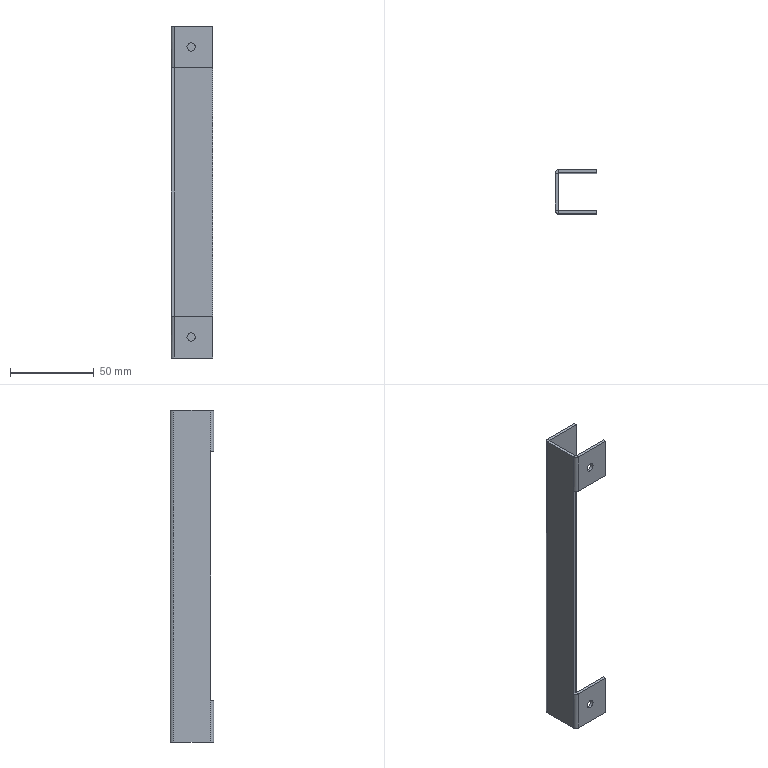Part | SolidWorks | features ICE 2, FlatPattern 1, SMBaseFlange 1, SheetMetal 1 | 1 solid | 34 faces | box 25 x 26 x 198 mm | volume 18838 mm3 | plane 26 | cylinder 8 | commonest cylinder face diameters 5 x4 0.4 x2 4 x2
STEP:
#1=CARTESIAN_POINT('',(-15.5,1.8,12.5));
#2=VERTEX_POINT('',#1);
#3=CARTESIAN_POINT('',(-10.5,1.8,12.5));
#4=VERTEX_POINT('',#3);
#5=CARTESIAN_POINT('',(-13.,1.8,12.5));
#6=DIRECTION('',(0.,-1.,0.));
#7=DIRECTION('',(1.,0.,0.));
#8=AXIS2_PLACEMENT_3D('',#5,#6,#7);
#9=CIRCLE('',#8,2.5);
#10=EDGE_CURVE('',#2,#4,#9,.T.);
#11=ORIENTED_EDGE('',*,*,#10,.F.);
#12=CARTESIAN_POINT('',(-15.5,0.,12.5));
#13=VERTEX_POINT('',#12);
#14=CARTESIAN_POINT('',(-15.5,10.,12.5));
#15=DIRECTION('',(0.,-1.,0.));
#16=VECTOR('',#15,1000.);
#17=LINE('',#14,#16);
#18=EDGE_CURVE('',#2,#13,#17,.T.);
#19=ORIENTED_EDGE('',*,*,#18,.T.);
#20=CARTESIAN_POINT('',(-10.5,0.,12.5));
#21=VERTEX_POINT('',#20);
#22=CARTESIAN_POINT('',(-13.,0.,12.5));
#23=DIRECTION('',(0.,-1.,0.));
#24=DIRECTION('',(1.,0.,0.));
#25=AXIS2_PLACEMENT_3D('',#22,#23,#24);
#26=CIRCLE('',#25,2.5);
#27=EDGE_CURVE('',#13,#21,#26,.T.);
#28=ORIENTED_EDGE('',*,*,#27,.T.);
#29=CARTESIAN_POINT('',(-10.5,10.,12.5));
#30=DIRECTION('',(0.,-1.,0.));
#31=VECTOR('',#30,1000.);
#32=LINE('',#29,#31);
#33=EDGE_CURVE('',#4,#21,#32,.T.);
#34=ORIENTED_EDGE('',*,*,#33,.F.);
#35=EDGE_LOOP('',(#11,#19,#28,#34));
#36=FACE_OUTER_BOUND('',#35,.T.);
#37=CARTESIAN_POINT('',(-13.,10.,12.5));
#38=DIRECTION('',(0.,-1.,0.));
#39=DIRECTION('',(1.,0.,0.));
#40=AXIS2_PLACEMENT_3D('',#37,#38,#39);
#41=CYLINDRICAL_SURFACE('',#40,2.5);
#42=ADVANCED_FACE('',(#36),#41,.F.);
#43=CARTESIAN_POINT('',(-15.5,1.8,185.5));
#44=VERTEX_POINT('',#43);
#45=CARTESIAN_POINT('',(-10.5,1.8,185.5));
#46=VERTEX_POINT('',#45);
#47=CARTESIAN_POINT('',(-13.,1.8,185.5));
#48=DIRECTION('',(0.,-1.,0.));
#49=DIRECTION('',(1.,0.,0.));
#50=AXIS2_PLACEMENT_3D('',#47,#48,#49);
#51=CIRCLE('',#50,2.5);
#52=EDGE_CURVE('',#44,#46,#51,.T.);
#53=ORIENTED_EDGE('',*,*,#52,.F.);
#54=CARTESIAN_POINT('',(-15.5,0.,185.5));
#55=VERTEX_POINT('',#54);
#56=CARTESIAN_POINT('',(-15.5,10.,185.5));
#57=DIRECTION('',(0.,-1.,0.));
#58=VECTOR('',#57,1000.);
#59=LINE('',#56,#58);
#60=EDGE_CURVE('',#44,#55,#59,.T.);
#61=ORIENTED_EDGE('',*,*,#60,.T.);
#62=CARTESIAN_POINT('',(-10.5,0.,185.5));
#63=VERTEX_POINT('',#62);
#64=CARTESIAN_POINT('',(-13.,0.,185.5));
#65=DIRECTION('',(0.,-1.,0.));
#66=DIRECTION('',(1.,0.,0.));
#67=AXIS2_PLACEMENT_3D('',#64,#65,#66);
#68=CIRCLE('',#67,2.5);
#69=EDGE_CURVE('',#55,#63,#68,.T.);
#70=ORIENTED_EDGE('',*,*,#69,.T.);
#71=CARTESIAN_POINT('',(-10.5,10.,185.5));
#72=DIRECTION('',(0.,-1.,0.));
#73=VECTOR('',#72,1000.);
#74=LINE('',#71,#73);
#75=EDGE_CURVE('',#46,#63,#74,.T.);
#76=ORIENTED_EDGE('',*,*,#75,.F.);
#77=EDGE_LOOP('',(#53,#61,#70,#76));
#78=FACE_OUTER_BOUND('',#77,.T.);
#79=CARTESIAN_POINT('',(-13.,10.,185.5));
#80=DIRECTION('',(0.,-1.,0.));
#81=DIRECTION('',(1.,0.,0.));
#82=AXIS2_PLACEMENT_3D('',#79,#80,#81);
#83=CYLINDRICAL_SURFACE('',#82,2.5);
#84=ADVANCED_FACE('',(#78),#83,.F.);
#85=CARTESIAN_POINT('',(-24.99,1.8,25.));
#86=VERTEX_POINT('',#85);
#87=CARTESIAN_POINT('',(-24.99,1.8,173.));
#88=VERTEX_POINT('',#87);
#89=CARTESIAN_POINT('',(-24.99,1.8,25.));
#90=DIRECTION('',(0.,0.,1.));
#91=VECTOR('',#90,1000.);
#92=LINE('',#89,#91);
#93=EDGE_CURVE('',#86,#88,#92,.T.);
#94=ORIENTED_EDGE('',*,*,#93,.T.);
#95=CARTESIAN_POINT('',(-23.,0.,173.));
#96=VERTEX_POINT('',#95);
#97=CARTESIAN_POINT('',(-23.,2.,173.));
#98=DIRECTION('',(0.,0.,1.));
#99=DIRECTION('',(1.,0.,0.));
#100=AXIS2_PLACEMENT_3D('',#97,#98,#99);
#101=CIRCLE('',#100,2.);
#102=EDGE_CURVE('',#88,#96,#101,.T.);
#103=ORIENTED_EDGE('',*,*,#102,.T.);
#104=CARTESIAN_POINT('',(-23.,0.,198.));
#105=VERTEX_POINT('',#104);
#106=CARTESIAN_POINT('',(-23.,0.,198.));
#107=DIRECTION('',(0.,0.,-1.));
#108=VECTOR('',#107,1000.);
#109=LINE('',#106,#108);
#110=EDGE_CURVE('',#105,#96,#109,.T.);
#111=ORIENTED_EDGE('',*,*,#110,.F.);
#112=CARTESIAN_POINT('',(-25.,2.,198.));
#113=VERTEX_POINT('',#112);
#114=CARTESIAN_POINT('',(-23.,2.,198.));
#115=DIRECTION('',(0.,0.,-1.));
#116=DIRECTION('',(1.,0.,0.));
#117=AXIS2_PLACEMENT_3D('',#114,#115,#116);
#118=CIRCLE('',#117,2.);
#119=EDGE_CURVE('',#105,#113,#118,.T.);
#120=ORIENTED_EDGE('',*,*,#119,.T.);
#121=CARTESIAN_POINT('',(-25.,2.,0.));
#122=VERTEX_POINT('',#121);
#123=CARTESIAN_POINT('',(-25.,2.,198.));
#124=DIRECTION('',(0.,0.,-1.));
#125=VECTOR('',#124,1000.);
#126=LINE('',#123,#125);
#127=EDGE_CURVE('',#113,#122,#126,.T.);
#128=ORIENTED_EDGE('',*,*,#127,.T.);
#129=CARTESIAN_POINT('',(-23.,0.,0.));
#130=VERTEX_POINT('',#129);
#131=CARTESIAN_POINT('',(-23.,2.,0.));
#132=DIRECTION('',(0.,0.,-1.));
#133=DIRECTION('',(1.,0.,0.));
#134=AXIS2_PLACEMENT_3D('',#131,#132,#133);
#135=CIRCLE('',#134,2.);
#136=EDGE_CURVE('',#130,#122,#135,.T.);
#137=ORIENTED_EDGE('',*,*,#136,.F.);
#138=CARTESIAN_POINT('',(-23.,0.,25.));
#139=VERTEX_POINT('',#138);
#140=CARTESIAN_POINT('',(-23.,0.,198.));
#141=DIRECTION('',(0.,0.,-1.));
#142=VECTOR('',#141,1000.);
#143=LINE('',#140,#142);
#144=EDGE_CURVE('',#139,#130,#143,.T.);
#145=ORIENTED_EDGE('',*,*,#144,.F.);
#146=CARTESIAN_POINT('',(-23.,2.,25.));
#147=DIRECTION('',(0.,0.,-1.));
#148=DIRECTION('',(-1.,0.,0.));
#149=AXIS2_PLACEMENT_3D('',#146,#147,#148);
#150=CIRCLE('',#149,2.);
#151=EDGE_CURVE('',#139,#86,#150,.T.);
#152=ORIENTED_EDGE('',*,*,#151,.T.);
#153=EDGE_LOOP('',(#94,#103,#111,#120,#128,#137,#145,#152));
#154=FACE_OUTER_BOUND('',#153,.T.);
#155=CARTESIAN_POINT('',(-23.,2.,198.));
#156=DIRECTION('',(0.,0.,-1.));
#157=DIRECTION('',(-1.,0.,0.));
#158=AXIS2_PLACEMENT_3D('',#155,#156,#157);
#159=CYLINDRICAL_SURFACE('',#158,2.);
#160=ADVANCED_FACE('',(#154),#159,.T.);
#161=CARTESIAN_POINT('',(-13.,0.,12.5));
#162=DIRECTION('',(0.,-1.,0.));
#163=DIRECTION('',(1.,0.,0.));
#164=AXIS2_PLACEMENT_3D('',#161,#162,#163);
#165=CIRCLE('',#164,2.5);
#166=EDGE_CURVE('',#21,#13,#165,.T.);
#167=ORIENTED_EDGE('',*,*,#166,.F.);
#168=ORIENTED_EDGE('',*,*,#27,.F.);
#169=EDGE_LOOP('',(#167,#168));
#170=FACE_BOUND('',#169,.T.);
#171=CARTESIAN_POINT('',(0.,0.,25.));
#172=VERTEX_POINT('',#171);
#173=CARTESIAN_POINT('',(0.,0.,0.));
#174=VERTEX_POINT('',#173);
#175=CARTESIAN_POINT('',(0.,0.,198.));
#176=DIRECTION('',(0.,0.,-1.));
#177=VECTOR('',#176,1000.);
#178=LINE('',#175,#177);
#179=EDGE_CURVE('',#172,#174,#178,.T.);
#180=ORIENTED_EDGE('',*,*,#179,.F.);
#181=CARTESIAN_POINT('',(45.,0.,25.));
#182=DIRECTION('',(1.,0.,0.));
#183=VECTOR('',#182,1000.);
#184=LINE('',#181,#183);
#185=EDGE_CURVE('',#139,#172,#184,.T.);
#186=ORIENTED_EDGE('',*,*,#185,.F.);
#187=ORIENTED_EDGE('',*,*,#144,.T.);
#188=CARTESIAN_POINT('',(0.,0.,0.));
#189=DIRECTION('',(-1.,0.,0.));
#190=VECTOR('',#189,1000.);
#191=LINE('',#188,#190);
#192=EDGE_CURVE('',#174,#130,#191,.T.);
#193=ORIENTED_EDGE('',*,*,#192,.F.);
#194=EDGE_LOOP('',(#180,#186,#187,#193));
#195=FACE_OUTER_BOUND('',#194,.T.);
#196=CARTESIAN_POINT('',(0.,0.,198.));
#197=DIRECTION('',(0.,-1.,0.));
#198=DIRECTION('',(1.,0.,0.));
#199=AXIS2_PLACEMENT_3D('',#196,#197,#198);
#200=PLANE('',#199);
#201=ADVANCED_FACE('',(#170,#195),#200,.T.);
#202=CARTESIAN_POINT('',(-13.,0.,185.5));
#203=DIRECTION('',(0.,-1.,0.));
#204=DIRECTION('',(1.,0.,0.));
#205=AXIS2_PLACEMENT_3D('',#202,#203,#204);
#206=CIRCLE('',#205,2.5);
#207=EDGE_CURVE('',#63,#55,#206,.T.);
#208=ORIENTED_EDGE('',*,*,#207,.F.);
#209=ORIENTED_EDGE('',*,*,#69,.F.);
#210=EDGE_LOOP('',(#208,#209));
#211=FACE_BOUND('',#210,.T.);
#212=ORIENTED_EDGE('',*,*,#110,.T.);
#213=CARTESIAN_POINT('',(0.,0.,173.));
#214=VERTEX_POINT('',#213);
#215=CARTESIAN_POINT('',(45.,0.,173.));
#216=DIRECTION('',(-1.,0.,0.));
#217=VECTOR('',#216,1000.);
#218=LINE('',#215,#217);
#219=EDGE_CURVE('',#214,#96,#218,.T.);
#220=ORIENTED_EDGE('',*,*,#219,.F.);
#221=CARTESIAN_POINT('',(0.,0.,198.));
#222=VERTEX_POINT('',#221);
#223=CARTESIAN_POINT('',(0.,0.,198.));
#224=DIRECTION('',(0.,0.,-1.));
#225=VECTOR('',#224,1000.);
#226=LINE('',#223,#225);
#227=EDGE_CURVE('',#222,#214,#226,.T.);
#228=ORIENTED_EDGE('',*,*,#227,.F.);
#229=CARTESIAN_POINT('',(0.,0.,198.));
#230=DIRECTION('',(-1.,0.,0.));
#231=VECTOR('',#230,1000.);
#232=LINE('',#229,#231);
#233=EDGE_CURVE('',#222,#105,#232,.T.);
#234=ORIENTED_EDGE('',*,*,#233,.T.);
#235=EDGE_LOOP('',(#212,#220,#228,#234));
#236=FACE_OUTER_BOUND('',#235,.T.);
#237=CARTESIAN_POINT('',(0.,0.,198.));
#238=DIRECTION('',(0.,-1.,0.));
#239=DIRECTION('',(1.,0.,0.));
#240=AXIS2_PLACEMENT_3D('',#237,#238,#239);
#241=PLANE('',#240);
#242=ADVANCED_FACE('',(#211,#236),#241,.T.);
#243=CARTESIAN_POINT('',(0.,1.8,25.));
#244=VERTEX_POINT('',#243);
#245=CARTESIAN_POINT('',(0.,1.8,0.));
#246=VERTEX_POINT('',#245);
#247=CARTESIAN_POINT('',(0.,1.8,198.));
#248=DIRECTION('',(0.,0.,-1.));
#249=VECTOR('',#248,1000.);
#250=LINE('',#247,#249);
#251=EDGE_CURVE('',#244,#246,#250,.T.);
#252=ORIENTED_EDGE('',*,*,#251,.F.);
#253=CARTESIAN_POINT('',(0.,0.,25.));
#254=DIRECTION('',(0.,1.,0.));
#255=VECTOR('',#254,1000.);
#256=LINE('',#253,#255);
#257=EDGE_CURVE('',#172,#244,#256,.T.);
#258=ORIENTED_EDGE('',*,*,#257,.F.);
#259=ORIENTED_EDGE('',*,*,#179,.T.);
#260=CARTESIAN_POINT('',(0.,1.8,0.));
#261=DIRECTION('',(0.,-1.,0.));
#262=VECTOR('',#261,1000.);
#263=LINE('',#260,#262);
#264=EDGE_CURVE('',#246,#174,#263,.T.);
#265=ORIENTED_EDGE('',*,*,#264,.F.);
#266=EDGE_LOOP('',(#252,#258,#259,#265));
#267=FACE_OUTER_BOUND('',#266,.T.);
#268=CARTESIAN_POINT('',(0.,1.8,198.));
#269=DIRECTION('',(1.,0.,0.));
#270=DIRECTION('',(0.,1.,0.));
#271=AXIS2_PLACEMENT_3D('',#268,#269,#270);
#272=PLANE('',#271);
#273=ADVANCED_FACE('',(#267),#272,.T.);
#274=ORIENTED_EDGE('',*,*,#227,.T.);
#275=CARTESIAN_POINT('',(0.,1.8,173.));
#276=VERTEX_POINT('',#275);
#277=CARTESIAN_POINT('',(0.,0.,173.));
#278=DIRECTION('',(0.,1.,0.));
#279=VECTOR('',#278,1000.);
#280=LINE('',#277,#279);
#281=EDGE_CURVE('',#214,#276,#280,.T.);
#282=ORIENTED_EDGE('',*,*,#281,.T.);
#283=CARTESIAN_POINT('',(0.,1.8,198.));
#284=VERTEX_POINT('',#283);
#285=CARTESIAN_POINT('',(0.,1.8,198.));
#286=DIRECTION('',(0.,0.,-1.));
#287=VECTOR('',#286,1000.);
#288=LINE('',#285,#287);
#289=EDGE_CURVE('',#284,#276,#288,.T.);
#290=ORIENTED_EDGE('',*,*,#289,.F.);
#291=CARTESIAN_POINT('',(0.,1.8,198.));
#292=DIRECTION('',(0.,-1.,0.));
#293=VECTOR('',#292,1000.);
#294=LINE('',#291,#293);
#295=EDGE_CURVE('',#284,#222,#294,.T.);
#296=ORIENTED_EDGE('',*,*,#295,.T.);
#297=EDGE_LOOP('',(#274,#282,#290,#296));
#298=FACE_OUTER_BOUND('',#297,.T.);
#299=CARTESIAN_POINT('',(0.,1.8,198.));
#300=DIRECTION('',(1.,0.,0.));
#301=DIRECTION('',(0.,1.,0.));
#302=AXIS2_PLACEMENT_3D('',#299,#300,#301);
#303=PLANE('',#302);
#304=ADVANCED_FACE('',(#298),#303,.T.);
#305=CARTESIAN_POINT('',(-13.,1.8,12.5));
#306=DIRECTION('',(0.,-1.,0.));
#307=DIRECTION('',(1.,0.,0.));
#308=AXIS2_PLACEMENT_3D('',#305,#306,#307);
#309=CIRCLE('',#308,2.5);
#310=EDGE_CURVE('',#4,#2,#309,.T.);
#311=ORIENTED_EDGE('',*,*,#310,.T.);
#312=ORIENTED_EDGE('',*,*,#10,.T.);
#313=EDGE_LOOP('',(#311,#312));
#314=FACE_BOUND('',#313,.T.);
#315=CARTESIAN_POINT('',(-23.,1.8,25.));
#316=VERTEX_POINT('',#315);
#317=CARTESIAN_POINT('',(0.,1.8,25.));
#318=DIRECTION('',(1.,0.,0.));
#319=VECTOR('',#318,1000.);
#320=LINE('',#317,#319);
#321=EDGE_CURVE('',#316,#244,#320,.T.);
#322=ORIENTED_EDGE('',*,*,#321,.T.);
#323=ORIENTED_EDGE('',*,*,#251,.T.);
#324=CARTESIAN_POINT('',(-23.,1.8,0.));
#325=VERTEX_POINT('',#324);
#326=CARTESIAN_POINT('',(0.,1.8,0.));
#327=DIRECTION('',(-1.,0.,0.));
#328=VECTOR('',#327,1000.);
#329=LINE('',#326,#328);
#330=EDGE_CURVE('',#246,#325,#329,.T.);
#331=ORIENTED_EDGE('',*,*,#330,.T.);
#332=CARTESIAN_POINT('',(-23.,1.8,198.));
#333=DIRECTION('',(0.,0.,-1.));
#334=VECTOR('',#333,1000.);
#335=LINE('',#332,#334);
#336=EDGE_CURVE('',#316,#325,#335,.T.);
#337=ORIENTED_EDGE('',*,*,#336,.F.);
#338=EDGE_LOOP('',(#322,#323,#331,#337));
#339=FACE_OUTER_BOUND('',#338,.T.);
#340=CARTESIAN_POINT('',(0.,1.8,198.));
#341=DIRECTION('',(0.,-1.,0.));
#342=DIRECTION('',(1.,0.,0.));
#343=AXIS2_PLACEMENT_3D('',#340,#341,#342);
#344=PLANE('',#343);
#345=ADVANCED_FACE('',(#314,#339),#344,.F.);
#346=CARTESIAN_POINT('',(-13.,1.8,185.5));
#347=DIRECTION('',(0.,-1.,0.));
#348=DIRECTION('',(1.,0.,0.));
#349=AXIS2_PLACEMENT_3D('',#346,#347,#348);
#350=CIRCLE('',#349,2.5);
#351=EDGE_CURVE('',#46,#44,#350,.T.);
#352=ORIENTED_EDGE('',*,*,#351,.T.);
#353=ORIENTED_EDGE('',*,*,#52,.T.);
#354=EDGE_LOOP('',(#352,#353));
#355=FACE_BOUND('',#354,.T.);
#356=CARTESIAN_POINT('',(-23.,1.8,173.));
#357=VERTEX_POINT('',#356);
#358=CARTESIAN_POINT('',(0.,1.8,173.));
#359=DIRECTION('',(-1.,0.,0.));
#360=VECTOR('',#359,1000.);
#361=LINE('',#358,#360);
#362=EDGE_CURVE('',#276,#357,#361,.T.);
#363=ORIENTED_EDGE('',*,*,#362,.T.);
#364=CARTESIAN_POINT('',(-23.,1.8,198.));
#365=VERTEX_POINT('',#364);
#366=CARTESIAN_POINT('',(-23.,1.8,198.));
#367=DIRECTION('',(0.,0.,-1.));
#368=VECTOR('',#367,1000.);
#369=LINE('',#366,#368);
#370=EDGE_CURVE('',#365,#357,#369,.T.);
#371=ORIENTED_EDGE('',*,*,#370,.F.);
#372=CARTESIAN_POINT('',(0.,1.8,198.));
#373=DIRECTION('',(-1.,0.,0.));
#374=VECTOR('',#373,1000.);
#375=LINE('',#372,#374);
#376=EDGE_CURVE('',#284,#365,#375,.T.);
#377=ORIENTED_EDGE('',*,*,#376,.F.);
#378=ORIENTED_EDGE('',*,*,#289,.T.);
#379=EDGE_LOOP('',(#363,#371,#377,#378));
#380=FACE_OUTER_BOUND('',#379,.T.);
#381=CARTESIAN_POINT('',(0.,1.8,198.));
#382=DIRECTION('',(0.,-1.,0.));
#383=DIRECTION('',(1.,0.,0.));
#384=AXIS2_PLACEMENT_3D('',#381,#382,#383);
#385=PLANE('',#384);
#386=ADVANCED_FACE('',(#355,#380),#385,.F.);
#387=CARTESIAN_POINT('',(-23.199,1.98,173.));
#388=VERTEX_POINT('',#387);
#389=CARTESIAN_POINT('',(-23.,2.,173.));
#390=DIRECTION('',(0.,0.,1.));
#391=DIRECTION('',(-1.,0.,0.));
#392=AXIS2_PLACEMENT_3D('',#389,#390,#391);
#393=CIRCLE('',#392,0.2);
#394=EDGE_CURVE('',#388,#357,#393,.T.);
#395=ORIENTED_EDGE('',*,*,#394,.F.);
#396=CARTESIAN_POINT('',(-23.199,1.98,25.));
#397=VERTEX_POINT('',#396);
#398=CARTESIAN_POINT('',(-23.199,1.98,210.51));
#399=DIRECTION('',(0.,0.,1.));
#400=VECTOR('',#399,1000.);
#401=LINE('',#398,#400);
#402=EDGE_CURVE('',#397,#388,#401,.T.);
#403=ORIENTED_EDGE('',*,*,#402,.F.);
#404=CARTESIAN_POINT('',(-23.,2.,25.));
#405=DIRECTION('',(0.,0.,-1.));
#406=DIRECTION('',(-1.,0.,0.));
#407=AXIS2_PLACEMENT_3D('',#404,#405,#406);
#408=CIRCLE('',#407,0.2);
#409=EDGE_CURVE('',#316,#397,#408,.T.);
#410=ORIENTED_EDGE('',*,*,#409,.F.);
#411=ORIENTED_EDGE('',*,*,#336,.T.);
#412=CARTESIAN_POINT('',(-23.2,2.,0.));
#413=VERTEX_POINT('',#412);
#414=CARTESIAN_POINT('',(-23.,2.,0.));
#415=DIRECTION('',(0.,0.,-1.));
#416=DIRECTION('',(1.,0.,0.));
#417=AXIS2_PLACEMENT_3D('',#414,#415,#416);
#418=CIRCLE('',#417,0.2);
#419=EDGE_CURVE('',#325,#413,#418,.T.);
#420=ORIENTED_EDGE('',*,*,#419,.T.);
#421=CARTESIAN_POINT('',(-23.2,2.,198.));
#422=VERTEX_POINT('',#421);
#423=CARTESIAN_POINT('',(-23.2,2.,198.));
#424=DIRECTION('',(0.,0.,-1.));
#425=VECTOR('',#424,1000.);
#426=LINE('',#423,#425);
#427=EDGE_CURVE('',#422,#413,#426,.T.);
#428=ORIENTED_EDGE('',*,*,#427,.F.);
#429=CARTESIAN_POINT('',(-23.,2.,198.));
#430=DIRECTION('',(0.,0.,-1.));
#431=DIRECTION('',(1.,0.,0.));
#432=AXIS2_PLACEMENT_3D('',#429,#430,#431);
#433=CIRCLE('',#432,0.2);
#434=EDGE_CURVE('',#365,#422,#433,.T.);
#435=ORIENTED_EDGE('',*,*,#434,.F.);
#436=ORIENTED_EDGE('',*,*,#370,.T.);
#437=EDGE_LOOP('',(#395,#403,#410,#411,#420,#428,#435,#436));
#438=FACE_OUTER_BOUND('',#437,.T.);
#439=CARTESIAN_POINT('',(-23.,2.,198.));
#440=DIRECTION('',(0.,0.,-1.));
#441=DIRECTION('',(-1.,0.,0.));
#442=AXIS2_PLACEMENT_3D('',#439,#440,#441);
#443=CYLINDRICAL_SURFACE('',#442,0.2);
#444=ADVANCED_FACE('',(#438),#443,.F.);
#445=CARTESIAN_POINT('',(-25.,2.,198.));
#446=DIRECTION('',(1.,0.,0.));
#447=VECTOR('',#446,1000.);
#448=LINE('',#445,#447);
#449=EDGE_CURVE('',#113,#422,#448,.T.);
#450=ORIENTED_EDGE('',*,*,#449,.F.);
#451=ORIENTED_EDGE('',*,*,#119,.F.);
#452=CARTESIAN_POINT('',(-23.,1.8,198.));
#453=DIRECTION('',(0.,-1.,0.));
#454=VECTOR('',#453,1000.);
#455=LINE('',#452,#454);
#456=EDGE_CURVE('',#365,#105,#455,.T.);
#457=ORIENTED_EDGE('',*,*,#456,.F.);
#458=ORIENTED_EDGE('',*,*,#434,.T.);
#459=EDGE_LOOP('',(#450,#451,#457,#458));
#460=FACE_OUTER_BOUND('',#459,.T.);
#461=CARTESIAN_POINT('',(-25.,2.,198.));
#462=DIRECTION('',(0.,0.,1.));
#463=DIRECTION('',(1.,0.,0.));
#464=AXIS2_PLACEMENT_3D('',#461,#462,#463);
#465=PLANE('',#464);
#466=ADVANCED_FACE('',(#460),#465,.T.);
#467=CARTESIAN_POINT('',(-25.,24.,198.));
#468=VERTEX_POINT('',#467);
#469=CARTESIAN_POINT('',(-25.,0.,198.));
#470=DIRECTION('',(0.,1.,0.));
#471=VECTOR('',#470,1000.);
#472=LINE('',#469,#471);
#473=EDGE_CURVE('',#113,#468,#472,.T.);
#474=ORIENTED_EDGE('',*,*,#473,.F.);
#475=ORIENTED_EDGE('',*,*,#449,.T.);
#476=CARTESIAN_POINT('',(-23.2,24.,198.));
#477=VERTEX_POINT('',#476);
#478=CARTESIAN_POINT('',(-23.2,0.,198.));
#479=DIRECTION('',(0.,1.,0.));
#480=VECTOR('',#479,1000.);
#481=LINE('',#478,#480);
#482=EDGE_CURVE('',#422,#477,#481,.T.);
#483=ORIENTED_EDGE('',*,*,#482,.T.);
#484=CARTESIAN_POINT('',(-23.2,24.,198.));
#485=DIRECTION('',(-1.,0.,0.));
#486=VECTOR('',#485,1000.);
#487=LINE('',#484,#486);
#488=EDGE_CURVE('',#477,#468,#487,.T.);
#489=ORIENTED_EDGE('',*,*,#488,.T.);
#490=EDGE_LOOP('',(#474,#475,#483,#489));
#491=FACE_OUTER_BOUND('',#490,.T.);
#492=CARTESIAN_POINT('',(-23.,1.8,198.));
#493=DIRECTION('',(0.,0.,1.));
#494=DIRECTION('',(1.,0.,0.));
#495=AXIS2_PLACEMENT_3D('',#492,#493,#494);
#496=PLANE('',#495);
#497=ADVANCED_FACE('',(#491),#496,.T.);
#498=CARTESIAN_POINT('',(-23.,0.,0.));
#499=DIRECTION('',(0.,1.,0.));
#500=VECTOR('',#499,1000.);
#501=LINE('',#498,#500);
#502=EDGE_CURVE('',#130,#325,#501,.T.);
#503=ORIENTED_EDGE('',*,*,#502,.F.);
#504=ORIENTED_EDGE('',*,*,#136,.T.);
#505=CARTESIAN_POINT('',(-23.2,2.,0.));
#506=DIRECTION('',(-1.,0.,0.));
#507=VECTOR('',#506,1000.);
#508=LINE('',#505,#507);
#509=EDGE_CURVE('',#413,#122,#508,.T.);
#510=ORIENTED_EDGE('',*,*,#509,.F.);
#511=ORIENTED_EDGE('',*,*,#419,.F.);
#512=EDGE_LOOP('',(#503,#504,#510,#511));
#513=FACE_OUTER_BOUND('',#512,.T.);
#514=CARTESIAN_POINT('',(-23.,0.,0.));
#515=DIRECTION('',(0.,0.,-1.));
#516=DIRECTION('',(-1.,0.,0.));
#517=AXIS2_PLACEMENT_3D('',#514,#515,#516);
#518=PLANE('',#517);
#519=ADVANCED_FACE('',(#513),#518,.T.);
#520=ORIENTED_EDGE('',*,*,#192,.T.);
#521=ORIENTED_EDGE('',*,*,#502,.T.);
#522=ORIENTED_EDGE('',*,*,#330,.F.);
#523=ORIENTED_EDGE('',*,*,#264,.T.);
#524=EDGE_LOOP('',(#520,#521,#522,#523));
#525=FACE_OUTER_BOUND('',#524,.T.);
#526=CARTESIAN_POINT('',(-23.2,2.,0.));
#527=DIRECTION('',(0.,0.,-1.));
#528=DIRECTION('',(-1.,0.,0.));
#529=AXIS2_PLACEMENT_3D('',#526,#527,#528);
#530=PLANE('',#529);
#531=ADVANCED_FACE('',(#525),#530,.T.);
#532=CARTESIAN_POINT('',(-23.,26.,198.));
#533=VERTEX_POINT('',#532);
#534=CARTESIAN_POINT('',(-23.,24.2,198.));
#535=VERTEX_POINT('',#534);
#536=CARTESIAN_POINT('',(-23.,26.,198.));
#537=DIRECTION('',(0.,-1.,0.));
#538=VECTOR('',#537,1000.);
#539=LINE('',#536,#538);
#540=EDGE_CURVE('',#533,#535,#539,.T.);
#541=ORIENTED_EDGE('',*,*,#540,.F.);
#542=CARTESIAN_POINT('',(-23.,24.,198.));
#543=DIRECTION('',(0.,0.,-1.));
#544=DIRECTION('',(1.,0.,0.));
#545=AXIS2_PLACEMENT_3D('',#542,#543,#544);
#546=CIRCLE('',#545,2.);
#547=EDGE_CURVE('',#468,#533,#546,.T.);
#548=ORIENTED_EDGE('',*,*,#547,.F.);
#549=ORIENTED_EDGE('',*,*,#488,.F.);
#550=CARTESIAN_POINT('',(-23.,24.,198.));
#551=DIRECTION('',(0.,0.,-1.));
#552=DIRECTION('',(1.,0.,0.));
#553=AXIS2_PLACEMENT_3D('',#550,#551,#552);
#554=CIRCLE('',#553,0.2);
#555=EDGE_CURVE('',#477,#535,#554,.T.);
#556=ORIENTED_EDGE('',*,*,#555,.T.);
#557=EDGE_LOOP('',(#541,#548,#549,#556));
#558=FACE_OUTER_BOUND('',#557,.T.);
#559=CARTESIAN_POINT('',(-23.,26.,198.));
#560=DIRECTION('',(0.,0.,1.));
#561=DIRECTION('',(1.,0.,0.));
#562=AXIS2_PLACEMENT_3D('',#559,#560,#561);
#563=PLANE('',#562);
#564=ADVANCED_FACE('',(#558),#563,.T.);
#565=CARTESIAN_POINT('',(0.,26.,198.));
#566=VERTEX_POINT('',#565);
#567=CARTESIAN_POINT('',(-25.,26.,198.));
#568=DIRECTION('',(1.,0.,0.));
#569=VECTOR('',#568,1000.);
#570=LINE('',#567,#569);
#571=EDGE_CURVE('',#533,#566,#570,.T.);
#572=ORIENTED_EDGE('',*,*,#571,.F.);
#573=ORIENTED_EDGE('',*,*,#540,.T.);
#574=CARTESIAN_POINT('',(0.,24.2,198.));
#575=VERTEX_POINT('',#574);
#576=CARTESIAN_POINT('',(-25.,24.2,198.));
#577=DIRECTION('',(1.,0.,0.));
#578=VECTOR('',#577,1000.);
#579=LINE('',#576,#578);
#580=EDGE_CURVE('',#535,#575,#579,.T.);
#581=ORIENTED_EDGE('',*,*,#580,.T.);
#582=CARTESIAN_POINT('',(0.,26.,198.));
#583=DIRECTION('',(0.,-1.,0.));
#584=VECTOR('',#583,1000.);
#585=LINE('',#582,#584);
#586=EDGE_CURVE('',#566,#575,#585,.T.);
#587=ORIENTED_EDGE('',*,*,#586,.F.);
#588=EDGE_LOOP('',(#572,#573,#581,#587));
#589=FACE_OUTER_BOUND('',#588,.T.);
#590=CARTESIAN_POINT('',(-23.2,24.,198.));
#591=DIRECTION('',(0.,0.,1.));
#592=DIRECTION('',(1.,0.,0.));
#593=AXIS2_PLACEMENT_3D('',#590,#591,#592);
#594=PLANE('',#593);
#595=ADVANCED_FACE('',(#589),#594,.T.);
#596=CARTESIAN_POINT('',(-25.,24.,0.));
#597=VERTEX_POINT('',#596);
#598=CARTESIAN_POINT('',(-23.2,24.,0.));
#599=VERTEX_POINT('',#598);
#600=CARTESIAN_POINT('',(-25.,24.,0.));
#601=DIRECTION('',(1.,0.,0.));
#602=VECTOR('',#601,1000.);
#603=LINE('',#600,#602);
#604=EDGE_CURVE('',#597,#599,#603,.T.);
#605=ORIENTED_EDGE('',*,*,#604,.F.);
#606=CARTESIAN_POINT('',(-23.,26.,0.));
#607=VERTEX_POINT('',#606);
#608=CARTESIAN_POINT('',(-23.,24.,0.));
#609=DIRECTION('',(0.,0.,-1.));
#610=DIRECTION('',(1.,0.,0.));
#611=AXIS2_PLACEMENT_3D('',#608,#609,#610);
#612=CIRCLE('',#611,2.);
#613=EDGE_CURVE('',#597,#607,#612,.T.);
#614=ORIENTED_EDGE('',*,*,#613,.T.);
#615=CARTESIAN_POINT('',(-23.,24.2,0.));
#616=VERTEX_POINT('',#615);
#617=CARTESIAN_POINT('',(-23.,24.2,0.));
#618=DIRECTION('',(0.,1.,0.));
#619=VECTOR('',#618,1000.);
#620=LINE('',#617,#619);
#621=EDGE_CURVE('',#616,#607,#620,.T.);
#622=ORIENTED_EDGE('',*,*,#621,.F.);
#623=CARTESIAN_POINT('',(-23.,24.,0.));
#624=DIRECTION('',(0.,0.,-1.));
#625=DIRECTION('',(1.,0.,0.));
#626=AXIS2_PLACEMENT_3D('',#623,#624,#625);
#627=CIRCLE('',#626,0.2);
#628=EDGE_CURVE('',#599,#616,#627,.T.);
#629=ORIENTED_EDGE('',*,*,#628,.F.);
#630=EDGE_LOOP('',(#605,#614,#622,#629));
#631=FACE_OUTER_BOUND('',#630,.T.);
#632=CARTESIAN_POINT('',(-25.,24.,0.));
#633=DIRECTION('',(0.,0.,-1.));
#634=DIRECTION('',(-1.,0.,0.));
#635=AXIS2_PLACEMENT_3D('',#632,#633,#634);
#636=PLANE('',#635);
#637=ADVANCED_FACE('',(#631),#636,.T.);
#638=CARTESIAN_POINT('',(-25.,0.,0.));
#639=DIRECTION('',(0.,1.,0.));
#640=VECTOR('',#639,1000.);
#641=LINE('',#638,#640);
#642=EDGE_CURVE('',#122,#597,#641,.T.);
#643=ORIENTED_EDGE('',*,*,#642,.T.);
#644=ORIENTED_EDGE('',*,*,#604,.T.);
#645=CARTESIAN_POINT('',(-23.2,0.,0.));
#646=DIRECTION('',(0.,1.,0.));
#647=VECTOR('',#646,1000.);
#648=LINE('',#645,#647);
#649=EDGE_CURVE('',#413,#599,#648,.T.);
#650=ORIENTED_EDGE('',*,*,#649,.F.);
#651=ORIENTED_EDGE('',*,*,#509,.T.);
#652=EDGE_LOOP('',(#643,#644,#650,#651));
#653=FACE_OUTER_BOUND('',#652,.T.);
#654=CARTESIAN_POINT('',(-23.,24.2,0.));
#655=DIRECTION('',(0.,0.,-1.));
#656=DIRECTION('',(-1.,0.,0.));
#657=AXIS2_PLACEMENT_3D('',#654,#655,#656);
#658=PLANE('',#657);
#659=ADVANCED_FACE('',(#653),#658,.T.);
#660=CARTESIAN_POINT('',(0.,24.2,0.));
#661=VERTEX_POINT('',#660);
#662=CARTESIAN_POINT('',(-25.,24.2,0.));
#663=DIRECTION('',(1.,0.,0.));
#664=VECTOR('',#663,1000.);
#665=LINE('',#662,#664);
#666=EDGE_CURVE('',#616,#661,#665,.T.);
#667=ORIENTED_EDGE('',*,*,#666,.T.);
#668=CARTESIAN_POINT('',(0.,24.2,198.));
#669=DIRECTION('',(0.,0.,-1.));
#670=VECTOR('',#669,1000.);
#671=LINE('',#668,#670);
#672=EDGE_CURVE('',#575,#661,#671,.T.);
#673=ORIENTED_EDGE('',*,*,#672,.F.);
#674=ORIENTED_EDGE('',*,*,#580,.F.);
#675=CARTESIAN_POINT('',(-23.,24.2,198.));
#676=DIRECTION('',(0.,0.,-1.));
#677=VECTOR('',#676,1000.);
#678=LINE('',#675,#677);
#679=EDGE_CURVE('',#535,#616,#678,.T.);
#680=ORIENTED_EDGE('',*,*,#679,.T.);
#681=EDGE_LOOP('',(#667,#673,#674,#680));
#682=FACE_OUTER_BOUND('',#681,.T.);
#683=CARTESIAN_POINT('',(-25.,24.2,198.));
#684=DIRECTION('',(0.,1.,0.));
#685=DIRECTION('',(-1.,0.,0.));
#686=AXIS2_PLACEMENT_3D('',#683,#684,#685);
#687=PLANE('',#686);
#688=ADVANCED_FACE('',(#682),#687,.F.);
#689=CARTESIAN_POINT('',(0.,26.,0.));
#690=VERTEX_POINT('',#689);
#691=CARTESIAN_POINT('',(0.,26.,0.));
#692=DIRECTION('',(0.,-1.,0.));
#693=VECTOR('',#692,1000.);
#694=LINE('',#691,#693);
#695=EDGE_CURVE('',#690,#661,#694,.T.);
#696=ORIENTED_EDGE('',*,*,#695,.F.);
#697=CARTESIAN_POINT('',(0.,26.,198.));
#698=DIRECTION('',(0.,0.,-1.));
#699=VECTOR('',#698,1000.);
#700=LINE('',#697,#699);
#701=EDGE_CURVE('',#566,#690,#700,.T.);
#702=ORIENTED_EDGE('',*,*,#701,.F.);
#703=ORIENTED_EDGE('',*,*,#586,.T.);
#704=ORIENTED_EDGE('',*,*,#672,.T.);
#705=EDGE_LOOP('',(#696,#702,#703,#704));
#706=FACE_OUTER_BOUND('',#705,.T.);
#707=CARTESIAN_POINT('',(0.,26.,198.));
#708=DIRECTION('',(1.,0.,0.));
#709=DIRECTION('',(0.,0.,-1.));
#710=AXIS2_PLACEMENT_3D('',#707,#708,#709);
#711=PLANE('',#710);
#712=ADVANCED_FACE('',(#706),#711,.T.);
#713=CARTESIAN_POINT('',(-25.,26.,0.));
#714=DIRECTION('',(1.,0.,0.));
#715=VECTOR('',#714,1000.);
#716=LINE('',#713,#715);
#717=EDGE_CURVE('',#607,#690,#716,.T.);
#718=ORIENTED_EDGE('',*,*,#717,.F.);
#719=CARTESIAN_POINT('',(-23.,26.,198.));
#720=DIRECTION('',(0.,0.,-1.));
#721=VECTOR('',#720,1000.);
#722=LINE('',#719,#721);
#723=EDGE_CURVE('',#533,#607,#722,.T.);
#724=ORIENTED_EDGE('',*,*,#723,.F.);
#725=ORIENTED_EDGE('',*,*,#571,.T.);
#726=ORIENTED_EDGE('',*,*,#701,.T.);
#727=EDGE_LOOP('',(#718,#724,#725,#726));
#728=FACE_OUTER_BOUND('',#727,.T.);
#729=CARTESIAN_POINT('',(-25.,26.,198.));
#730=DIRECTION('',(0.,1.,0.));
#731=DIRECTION('',(-1.,0.,0.));
#732=AXIS2_PLACEMENT_3D('',#729,#730,#731);
#733=PLANE('',#732);
#734=ADVANCED_FACE('',(#728),#733,.T.);
#735=ORIENTED_EDGE('',*,*,#613,.F.);
#736=CARTESIAN_POINT('',(-25.,24.,198.));
#737=DIRECTION('',(0.,0.,-1.));
#738=VECTOR('',#737,1000.);
#739=LINE('',#736,#738);
#740=EDGE_CURVE('',#468,#597,#739,.T.);
#741=ORIENTED_EDGE('',*,*,#740,.F.);
#742=ORIENTED_EDGE('',*,*,#547,.T.);
#743=ORIENTED_EDGE('',*,*,#723,.T.);
#744=EDGE_LOOP('',(#735,#741,#742,#743));
#745=FACE_OUTER_BOUND('',#744,.T.);
#746=CARTESIAN_POINT('',(-23.,24.,198.));
#747=DIRECTION('',(0.,0.,-1.));
#748=DIRECTION('',(-1.,0.,0.));
#749=AXIS2_PLACEMENT_3D('',#746,#747,#748);
#750=CYLINDRICAL_SURFACE('',#749,2.);
#751=ADVANCED_FACE('',(#745),#750,.T.);
#752=ORIENTED_EDGE('',*,*,#642,.F.);
#753=ORIENTED_EDGE('',*,*,#127,.F.);
#754=ORIENTED_EDGE('',*,*,#473,.T.);
#755=ORIENTED_EDGE('',*,*,#740,.T.);
#756=EDGE_LOOP('',(#752,#753,#754,#755));
#757=FACE_OUTER_BOUND('',#756,.T.);
#758=CARTESIAN_POINT('',(-25.,0.,198.));
#759=DIRECTION('',(-1.,0.,0.));
#760=DIRECTION('',(0.,0.,1.));
#761=AXIS2_PLACEMENT_3D('',#758,#759,#760);
#762=PLANE('',#761);
#763=ADVANCED_FACE('',(#757),#762,.T.);
#764=ORIENTED_EDGE('',*,*,#649,.T.);
#765=CARTESIAN_POINT('',(-23.2,24.,198.));
#766=DIRECTION('',(0.,0.,-1.));
#767=VECTOR('',#766,1000.);
#768=LINE('',#765,#767);
#769=EDGE_CURVE('',#477,#599,#768,.T.);
#770=ORIENTED_EDGE('',*,*,#769,.F.);
#771=ORIENTED_EDGE('',*,*,#482,.F.);
#772=ORIENTED_EDGE('',*,*,#427,.T.);
#773=EDGE_LOOP('',(#764,#770,#771,#772));
#774=FACE_OUTER_BOUND('',#773,.T.);
#775=CARTESIAN_POINT('',(-23.2,0.,198.));
#776=DIRECTION('',(-1.,0.,0.));
#777=DIRECTION('',(0.,0.,1.));
#778=AXIS2_PLACEMENT_3D('',#775,#776,#777);
#779=PLANE('',#778);
#780=ADVANCED_FACE('',(#774),#779,.F.);
#781=ORIENTED_EDGE('',*,*,#628,.T.);
#782=ORIENTED_EDGE('',*,*,#679,.F.);
#783=ORIENTED_EDGE('',*,*,#555,.F.);
#784=ORIENTED_EDGE('',*,*,#769,.T.);
#785=EDGE_LOOP('',(#781,#782,#783,#784));
#786=FACE_OUTER_BOUND('',#785,.T.);
#787=CARTESIAN_POINT('',(-23.,24.,198.));
#788=DIRECTION('',(0.,0.,-1.));
#789=DIRECTION('',(-1.,0.,0.));
#790=AXIS2_PLACEMENT_3D('',#787,#788,#789);
#791=CYLINDRICAL_SURFACE('',#790,0.2);
#792=ADVANCED_FACE('',(#786),#791,.F.);
#793=ORIENTED_EDGE('',*,*,#376,.T.);
#794=ORIENTED_EDGE('',*,*,#456,.T.);
#795=ORIENTED_EDGE('',*,*,#233,.F.);
#796=ORIENTED_EDGE('',*,*,#295,.F.);
#797=EDGE_LOOP('',(#793,#794,#795,#796));
#798=FACE_OUTER_BOUND('',#797,.T.);
#799=CARTESIAN_POINT('',(-23.,24.,198.));
#800=DIRECTION('',(0.,0.,1.));
#801=DIRECTION('',(1.,0.,0.));
#802=AXIS2_PLACEMENT_3D('',#799,#800,#801);
#803=PLANE('',#802);
#804=ADVANCED_FACE('',(#798),#803,.T.);
#805=ORIENTED_EDGE('',*,*,#666,.F.);
#806=ORIENTED_EDGE('',*,*,#621,.T.);
#807=ORIENTED_EDGE('',*,*,#717,.T.);
#808=ORIENTED_EDGE('',*,*,#695,.T.);
#809=EDGE_LOOP('',(#805,#806,#807,#808));
#810=FACE_OUTER_BOUND('',#809,.T.);
#811=CARTESIAN_POINT('',(-23.,24.,0.));
#812=DIRECTION('',(0.,0.,1.));
#813=DIRECTION('',(1.,0.,0.));
#814=AXIS2_PLACEMENT_3D('',#811,#812,#813);
#815=PLANE('',#814);
#816=ADVANCED_FACE('',(#810),#815,.F.);
#817=CARTESIAN_POINT('',(-23.,0.,25.));
#818=DIRECTION('',(0.,1.,0.));
#819=VECTOR('',#818,1000.);
#820=LINE('',#817,#819);
#821=EDGE_CURVE('',#139,#316,#820,.T.);
#822=ORIENTED_EDGE('',*,*,#821,.F.);
#823=ORIENTED_EDGE('',*,*,#185,.T.);
#824=ORIENTED_EDGE('',*,*,#257,.T.);
#825=ORIENTED_EDGE('',*,*,#321,.F.);
#826=EDGE_LOOP('',(#822,#823,#824,#825));
#827=FACE_OUTER_BOUND('',#826,.T.);
#828=CARTESIAN_POINT('',(45.,0.,25.));
#829=DIRECTION('',(0.,0.,-1.));
#830=DIRECTION('',(1.,0.,0.));
#831=AXIS2_PLACEMENT_3D('',#828,#829,#830);
#832=PLANE('',#831);
#833=ADVANCED_FACE('',(#827),#832,.F.);
#834=ORIENTED_EDGE('',*,*,#219,.T.);
#835=CARTESIAN_POINT('',(-23.,0.,173.));
#836=DIRECTION('',(0.,1.,0.));
#837=VECTOR('',#836,1000.);
#838=LINE('',#835,#837);
#839=EDGE_CURVE('',#96,#357,#838,.T.);
#840=ORIENTED_EDGE('',*,*,#839,.T.);
#841=ORIENTED_EDGE('',*,*,#362,.F.);
#842=ORIENTED_EDGE('',*,*,#281,.F.);
#843=EDGE_LOOP('',(#834,#840,#841,#842));
#844=FACE_OUTER_BOUND('',#843,.T.);
#845=CARTESIAN_POINT('',(45.,0.,173.));
#846=DIRECTION('',(0.,0.,1.));
#847=DIRECTION('',(-1.,0.,0.));
#848=AXIS2_PLACEMENT_3D('',#845,#846,#847);
#849=PLANE('',#848);
#850=ADVANCED_FACE('',(#844),#849,.F.);
#851=CARTESIAN_POINT('',(-24.99,1.8,173.));
#852=DIRECTION('',(-0.995,-0.1,0.));
#853=VECTOR('',#852,1000.);
#854=LINE('',#851,#853);
#855=EDGE_CURVE('',#388,#88,#854,.T.);
#856=ORIENTED_EDGE('',*,*,#855,.F.);
#857=ORIENTED_EDGE('',*,*,#394,.T.);
#858=ORIENTED_EDGE('',*,*,#839,.F.);
#859=ORIENTED_EDGE('',*,*,#102,.F.);
#860=EDGE_LOOP('',(#856,#857,#858,#859));
#861=FACE_OUTER_BOUND('',#860,.T.);
#862=CARTESIAN_POINT('',(-23.,2.,173.));
#863=DIRECTION('',(0.,0.,-1.));
#864=DIRECTION('',(-1.,0.,0.));
#865=AXIS2_PLACEMENT_3D('',#862,#863,#864);
#866=PLANE('',#865);
#867=ADVANCED_FACE('',(#861),#866,.T.);
#868=CARTESIAN_POINT('',(-24.99,1.8,25.));
#869=DIRECTION('',(-0.995,-0.1,0.));
#870=VECTOR('',#869,1000.);
#871=LINE('',#868,#870);
#872=EDGE_CURVE('',#397,#86,#871,.T.);
#873=ORIENTED_EDGE('',*,*,#872,.F.);
#874=ORIENTED_EDGE('',*,*,#402,.T.);
#875=ORIENTED_EDGE('',*,*,#855,.T.);
#876=ORIENTED_EDGE('',*,*,#93,.F.);
#877=EDGE_LOOP('',(#873,#874,#875,#876));
#878=FACE_OUTER_BOUND('',#877,.T.);
#879=CARTESIAN_POINT('',(-24.99,1.8,99.));
#880=DIRECTION('',(0.1,-0.995,0.));
#881=DIRECTION('',(0.,0.,1.));
#882=AXIS2_PLACEMENT_3D('',#879,#880,#881);
#883=PLANE('',#882);
#884=ADVANCED_FACE('',(#878),#883,.T.);
#885=ORIENTED_EDGE('',*,*,#821,.T.);
#886=ORIENTED_EDGE('',*,*,#409,.T.);
#887=ORIENTED_EDGE('',*,*,#872,.T.);
#888=ORIENTED_EDGE('',*,*,#151,.F.);
#889=EDGE_LOOP('',(#885,#886,#887,#888));
#890=FACE_OUTER_BOUND('',#889,.T.);
#891=CARTESIAN_POINT('',(-23.,2.,25.));
#892=DIRECTION('',(0.,0.,1.));
#893=DIRECTION('',(1.,0.,0.));
#894=AXIS2_PLACEMENT_3D('',#891,#892,#893);
#895=PLANE('',#894);
#896=ADVANCED_FACE('',(#890),#895,.T.);
#897=ORIENTED_EDGE('',*,*,#60,.F.);
#898=ORIENTED_EDGE('',*,*,#351,.F.);
#899=ORIENTED_EDGE('',*,*,#75,.T.);
#900=ORIENTED_EDGE('',*,*,#207,.T.);
#901=EDGE_LOOP('',(#897,#898,#899,#900));
#902=FACE_OUTER_BOUND('',#901,.T.);
#903=CARTESIAN_POINT('',(-13.,10.,185.5));
#904=DIRECTION('',(0.,-1.,0.));
#905=DIRECTION('',(1.,0.,0.));
#906=AXIS2_PLACEMENT_3D('',#903,#904,#905);
#907=CYLINDRICAL_SURFACE('',#906,2.5);
#908=ADVANCED_FACE('',(#902),#907,.F.);
#909=ORIENTED_EDGE('',*,*,#18,.F.);
#910=ORIENTED_EDGE('',*,*,#310,.F.);
#911=ORIENTED_EDGE('',*,*,#33,.T.);
#912=ORIENTED_EDGE('',*,*,#166,.T.);
#913=EDGE_LOOP('',(#909,#910,#911,#912));
#914=FACE_OUTER_BOUND('',#913,.T.);
#915=CARTESIAN_POINT('',(-13.,10.,12.5));
#916=DIRECTION('',(0.,-1.,0.));
#917=DIRECTION('',(1.,0.,0.));
#918=AXIS2_PLACEMENT_3D('',#915,#916,#917);
#919=CYLINDRICAL_SURFACE('',#918,2.5);
#920=ADVANCED_FACE('',(#914),#919,.F.);
#921=CLOSED_SHELL('',(#42,#84,#160,#201,#242,#273,#304,#345,#386,#444,#466,#497,#519,#531,#564,#595,#637,#659,#688,#712,#734,#751,#763,#780,#792,#804,#816,#833,#850,#867,#884,#896,#908,#920));
#922=MANIFOLD_SOLID_BREP('',#921);
#923=CARTESIAN_POINT('',(0.,0.,0.));
#924=DIRECTION('',(0.,0.,1.));
#925=DIRECTION('',(1.,0.,0.));
#926=AXIS2_PLACEMENT_3D('',#923,#924,#925);
#927=(LENGTH_UNIT()NAMED_UNIT(*)SI_UNIT(.MILLI.,.METRE.));
#928=UNCERTAINTY_MEASURE_WITH_UNIT(LENGTH_MEASURE(0.00001),#927,'','');
#929=(NAMED_UNIT(*)PLANE_ANGLE_UNIT()SI_UNIT($,.RADIAN.));
#930=(NAMED_UNIT(*)SI_UNIT($,.STERADIAN.)SOLID_ANGLE_UNIT());
#931=(GEOMETRIC_REPRESENTATION_CONTEXT(3)GLOBAL_UNCERTAINTY_ASSIGNED_CONTEXT((#928))GLOBAL_UNIT_ASSIGNED_CONTEXT((#927,#929,#930))REPRESENTATION_CONTEXT('',''));
#932=ADVANCED_BREP_SHAPE_REPRESENTATION('',(#922,#926),#931);